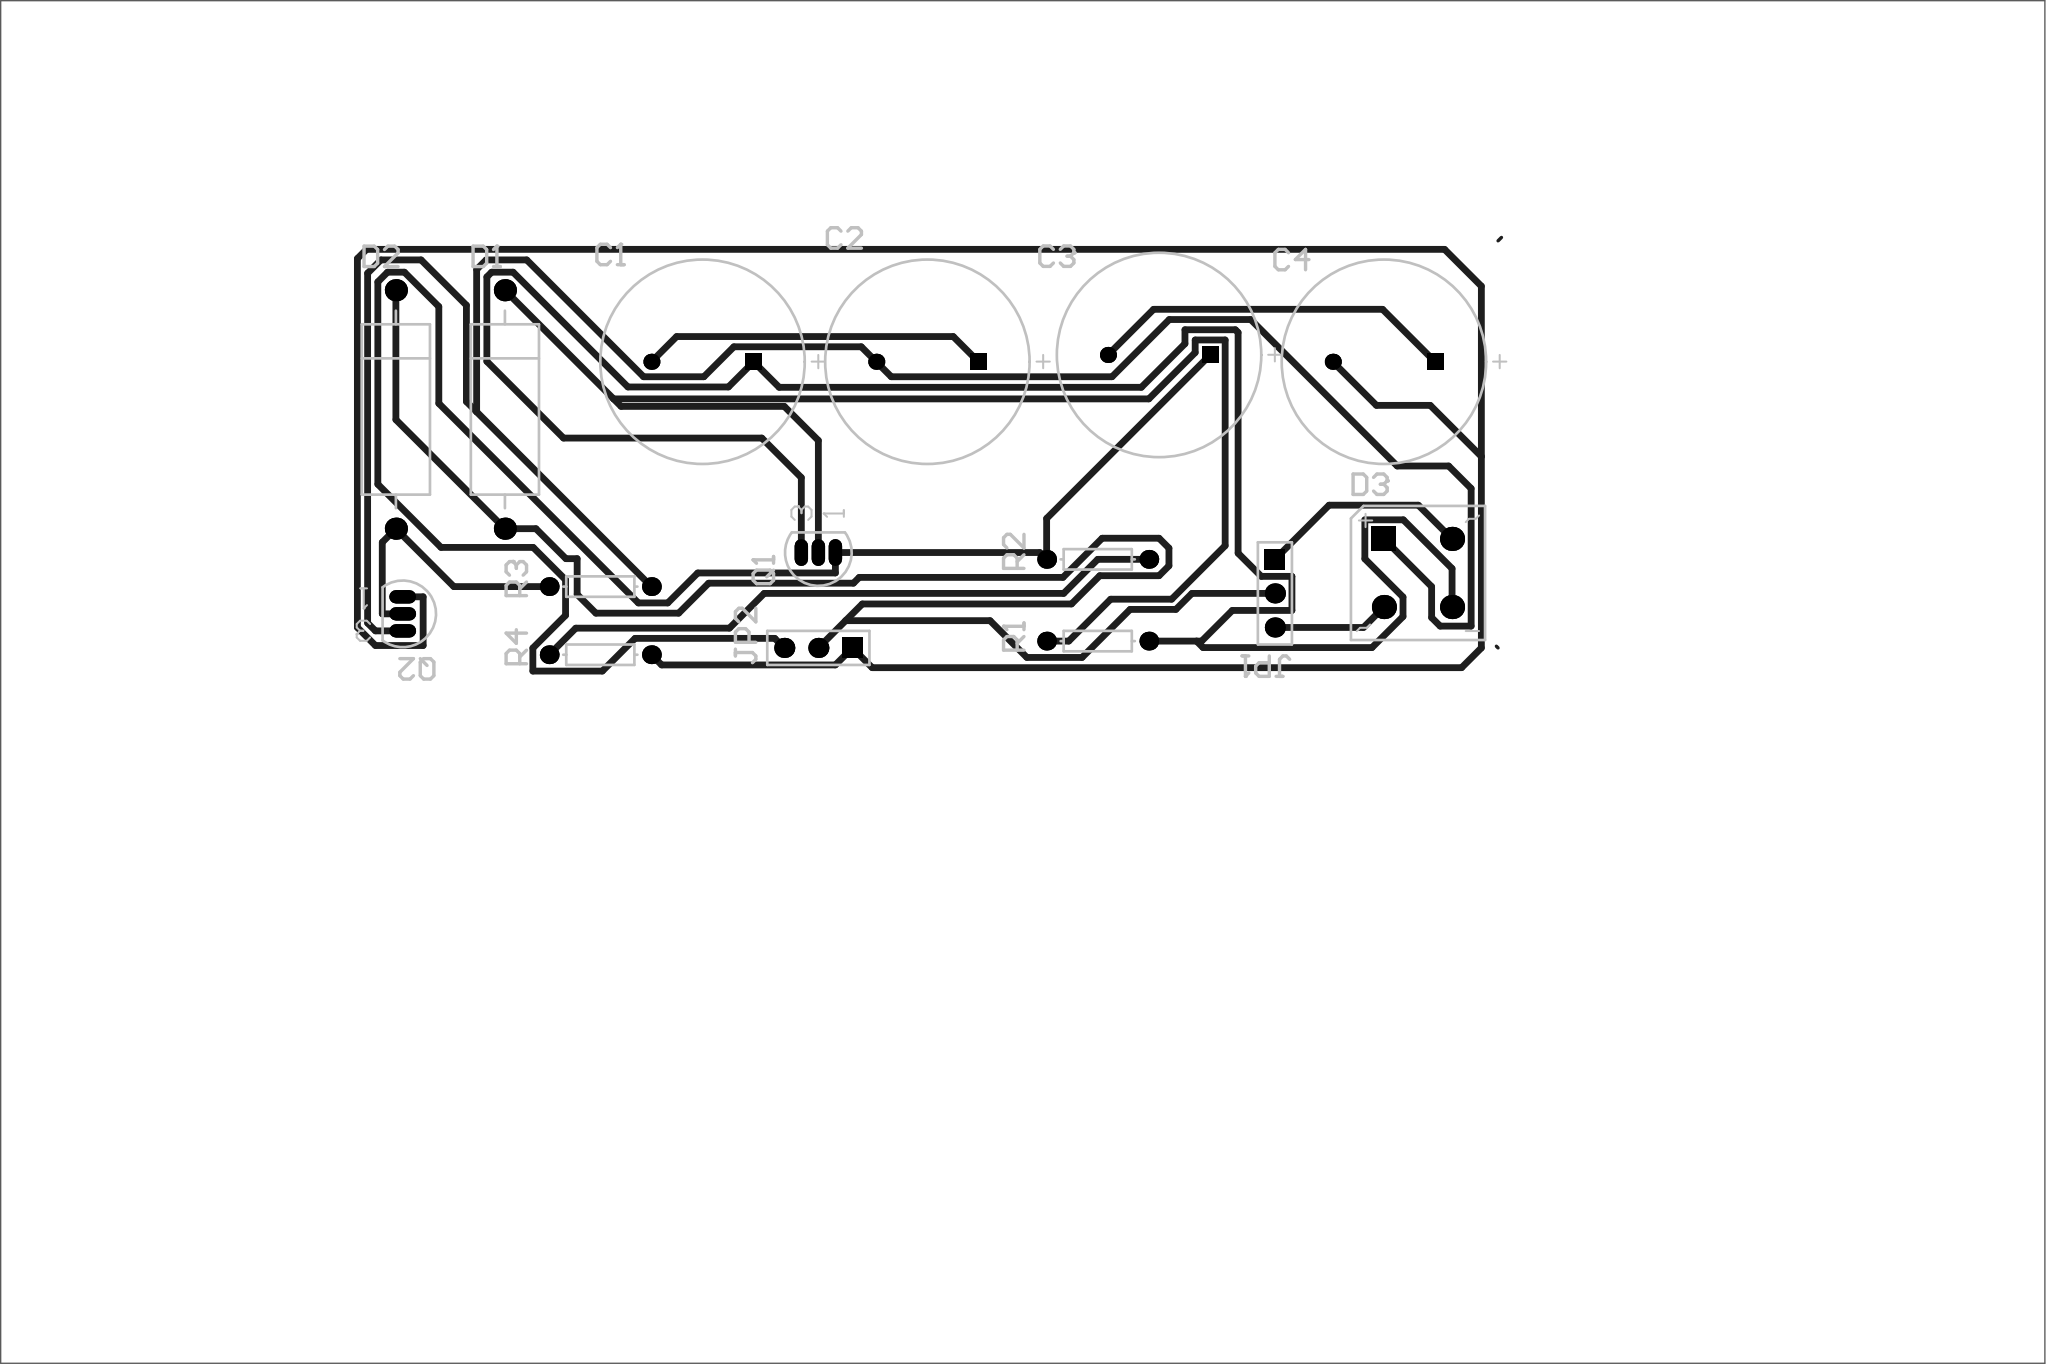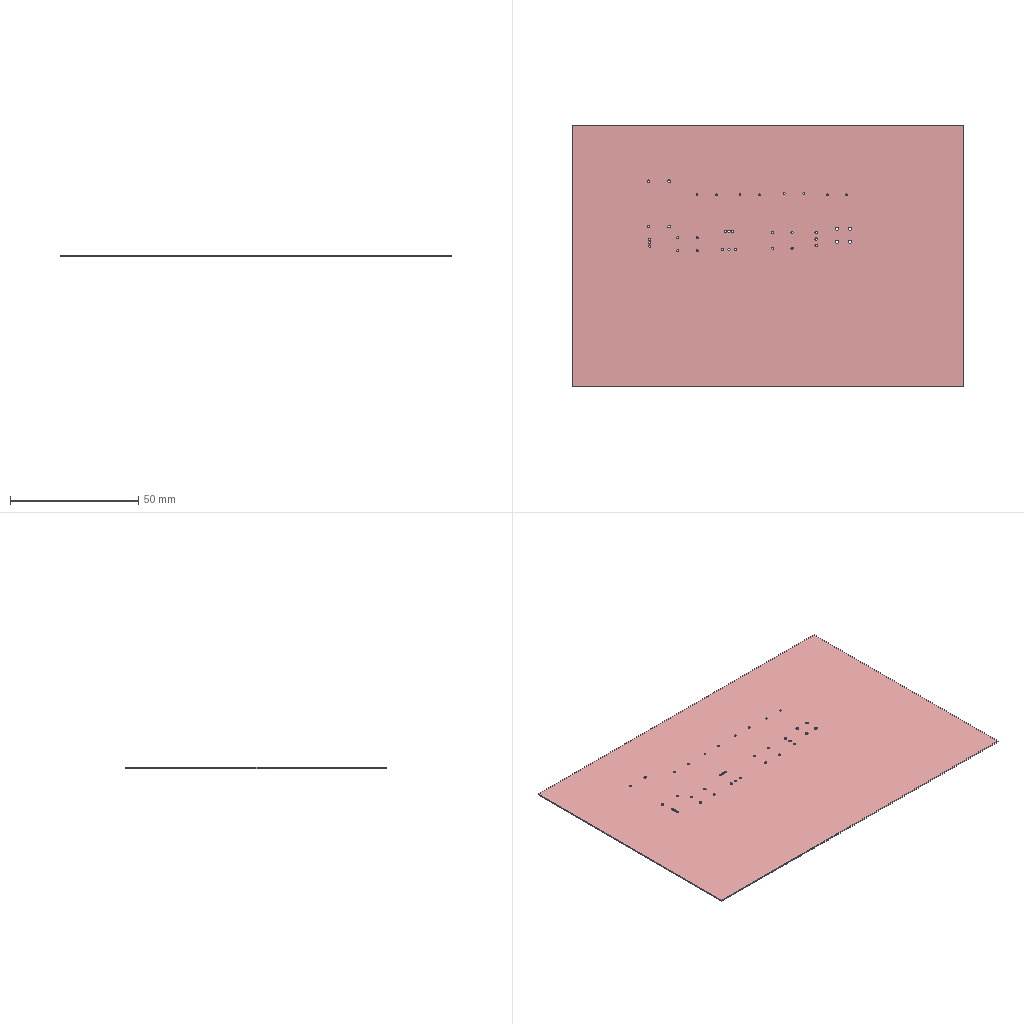Circuit board layout | Altium Designer | box 152.4 x 101.6 x 0.4 mm
Layer stack:
# Altium Designer layer stack of  (unit mm; dielectric type: 0 none, 1 core, 2 prepreg, 3 surface material)
index,name,kind,layer,copper_thickness_mm,dielectric_type,dielectric_thickness_mm,dielectric_material,dielectric_constant
0,Top Paste,other,,,,,,
1,Top Overlay,other,,,,,,
2,Top Solder,dielectric,,,3,0.0102,Solder Resist,3.5
3,Top Layer,copper,Top Layer,0.0356,,,,
4,Dielectric1,dielectric,,,0,0.32,FR-4,4.8
5,Bottom Layer,copper,Bottom Layer,0.0356,,,,
6,Bottom Solder,dielectric,,,3,0.0102,Solder Resist,3.5
7,Bottom Overlay,other,,,,,,
8,Bottom Paste,other,,,,,,
# drill layer pairs: low layer,high layer
drill_pair,Top Layer,Bottom Layer
Part placement:
Designator,Comment,Layer,Footprint,Center-X(mm),Center-Y(mm),Rotation
R4,Res1,TopLayer,AXIAL-0.3,70.104,78.232,180
R3,Res1,TopLayer,AXIAL-0.3,70.104,83.312,180
R2,Res1,TopLayer,AXIAL-0.3,107.188,85.344,180
R1,Res1,TopLayer,AXIAL-0.3,107.188,79.248,180
Q2,2N3906,TopLayer,BCY-W3/E4,55.372,81.28,180
Q1,2N3904,TopLayer,BCY-W3/E4,86.36,85.852,90
JP2,Header 3,TopLayer,HDR1X3,86.36,78.74,180
JP1,Header 3,TopLayer,HDR1X3,120.396,82.804,270
D3,Bridge1,TopLayer,E-BIP-P4/D10,131.064,84.328,0
D2,IN4736,TopLayer,DIODE-0.7,54.864,96.52,90
D1,IN4736,TopLayer,DIODE-0.7,62.992,96.52,90
C4,Cap Pol1,TopLayer,RB7.6-15,128.524,100.076,0
C3,Cap Pol1,TopLayer,RB7.6-15,111.76,100.584,0
C2,Cap Pol1,TopLayer,RB7.6-15,94.488,100.076,0
C1,Cap Pol1,TopLayer,RB7.6-15,77.724,100.076,0
Pad and via stacks:
# Altium Designer via and pad stacks of  (unit mm). Each distinct definition once, with the count of objects using it.
# via: kind,start_layer,end_layer,hole_mm,diameter_mm,mode(0 simple;1 top-mid-bottom;2 full stack),diameter_per_layer,count,example_net
# pad: kind,layer,hole_mm,hole_type(0 round;1 square;2 slot),plating,top_size,top_shape(1 round;2 rect;3 octagon;9 rounded rect),mid_size,bottom_size,mode,footprint,size_per_layer,count,example
pad,Multi-Layer,0.9,0,plated,2x1,1,2x1,2x1,0,BCY-W3/E4,,6,Q1.3
pad,Multi-Layer,0.85,0,plated,1.4x1.4,1,1.4x1.4,1.4x1.4,0,AXIAL-0.3,,8,R1.1
pad,Multi-Layer,1.2,0,plated,1.8x1.8,2,1.8x1.8,1.8x1.8,0,E-BIP-P4/D10,,1,D3.1
pad,Multi-Layer,1.2,0,plated,1.8x1.8,1,1.8x1.8,1.8x1.8,0,E-BIP-P4/D10,,3,D3.4
pad,Multi-Layer,0.9,0,plated,1.5x1.5,1,1.5x1.5,1.5x1.5,0,HDR1X3,,4,JP1.3
pad,Multi-Layer,0.9,0,plated,1.5x1.5,2,1.5x1.5,1.5x1.5,0,HDR1X3,,2,JP1.1
pad,Multi-Layer,0.7,0,plated,1.2x1.2,1,1.2x1.2,1.2x1.2,0,RB7.6-15,,4,C3.2
pad,Multi-Layer,0.7,0,plated,1.2x1.2,2,1.2x1.2,1.2x1.2,0,RB7.6-15,,4,C3.1
pad,Multi-Layer,1,0,plated,1.65x1.65,1,1.65x1.65,1.65x1.65,0,DIODE-0.7,,4,D1.1
Design rules, without the lines most boards share:
# Altium Designer design rules of  (exported by Altium Designer, unit mm)
# columns: name | kind | enabled | priority | scope1 | scope2 | descriptor | typed fields (field=value)
HoleToHoleClearance | 52 | enabled | 1 | All | All | Hole To Hole Clearance (Gap=10mil) (All),(All) | gap=0.254
DiffPairsRouting | 51 | enabled | 1 | All | All | Differential Pairs Uncoupled Length using the Gap Constraints (Min=10mil) (Max=10mil) (Prefered=10mil)  and Width Constraints (Min=15mil) (Max=15mil) (Prefered=15mil) (All) |
buxian | 9 | enabled | 1 | All | All | Routing Layers(All) |
Width Rules | 2 | enabled | 1 | All | All | Width Constraint (Min=20mil) (Max=20mil) (Preferred=20mil) (All) |
RoutingLayers | 9 | enabled | 2 | All | All | Routing Layers(All) |
Testpoint | 43 | enabled | 1 | All | All | Fabrication Testpoint Style (Under Component=Yes) (All) |
TestPointUsage | 44 | enabled | 1 | All | All | Fabrication Testpoint Usage (Valid =One Required, Allow multiple per net=No) (All) |
SolderMaskExpansion | 13 | enabled | 1 | All | All | Solder Mask Expansion (Expansion =4mil) (All) | expansion=0.1016
PasteMaskExpansion | 14 | enabled | 1 | All | All | Paste Mask Expansion (Expansion =0mil) (All) | expansion=0
RoutingVias | 11 | enabled | 1 | All | All | Routing Via (MinHoleWidth=28mil) (MaxHoleWidth=28mil) (PreferredHoleWidth=28mil) (MinWidth=50mil) (MaxWidth=50mil) (PreferedWidth=50mil) (All) | via_min_hole=0.7112 via_max_hole=0.7112 via_preferred_diameter=1.27 via_preferred_hole=0.7112
PolygonConnect | 20 | enabled | 1 | All | All | Polygon Connect Rule(Relief Connect )(Conductor Width=10mil) (Relief Angle=90 Angle) (Entries=4) (Air Gap Width=10mil) (All),(All) | connect_style(0=relief,1=direct,2=none)=0 relief_conductor_width=0.254 relief_entries=4
PlaneConnect | 6 | enabled | 1 | All | All | Power Plane Connect Rule(Relief Connect )(Expansion=20mil) (Conductor Width=10mil) (Air Gap=10mil) (Entries=4) (All) | relief_conductor_width=0.254 relief_entries=4 relief_expansion=0.508
Clearance | 0 | enabled | 1 | All | All | Clearance Constraint (Gap=10mil) (All),(All) | gap=0.254